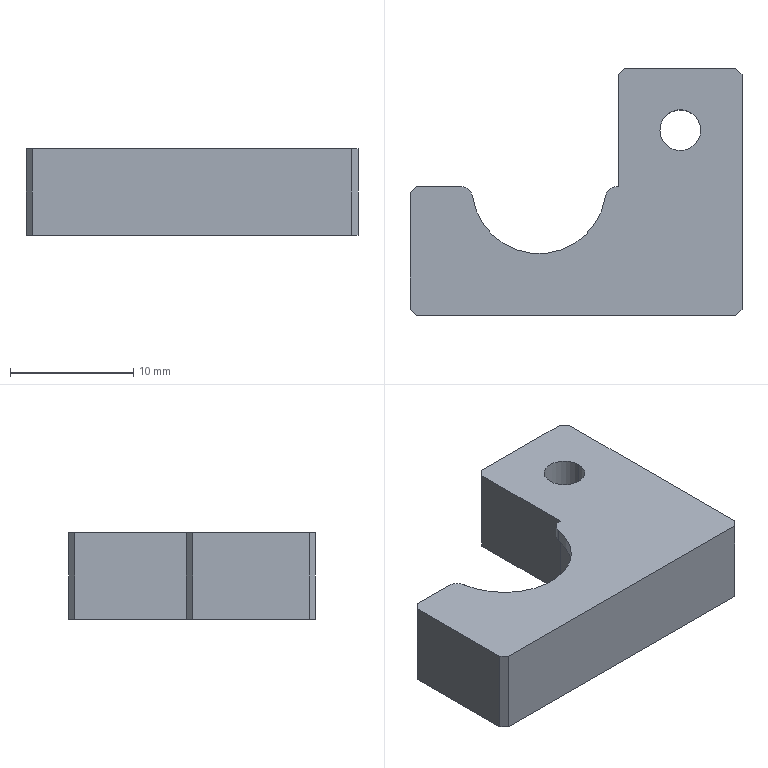Part | SolidWorks | features Chamfer 1, Extrusion 1, Fillet 1, HoleWzd 1, ICE 1 | 1 solid | 22 faces | box 26.9 x 20 x 7 mm | volume 2132 mm3 | plane 16 | cylinder 6 | commonest cylinder face diameters 2 x2 3.3 x2 10.9 x1 12.9 x1
STEP:
#1=CARTESIAN_POINT('',(9.8,4.55,0.));
#2=VERTEX_POINT('',#1);
#3=CARTESIAN_POINT('',(13.1,4.55,0.));
#4=VERTEX_POINT('',#3);
#5=CARTESIAN_POINT('',(11.45,4.55,0.));
#6=DIRECTION('',(0.,0.,1.));
#7=DIRECTION('',(1.,0.,0.));
#8=AXIS2_PLACEMENT_3D('',#5,#6,#7);
#9=CIRCLE('',#8,1.65);
#10=EDGE_CURVE('',#2,#4,#9,.T.);
#11=ORIENTED_EDGE('',*,*,#10,.F.);
#12=CARTESIAN_POINT('',(9.8,4.55,7.));
#13=VERTEX_POINT('',#12);
#14=CARTESIAN_POINT('',(9.8,4.55,7.));
#15=DIRECTION('',(0.,0.,1.));
#16=VECTOR('',#15,1000.);
#17=LINE('',#14,#16);
#18=EDGE_CURVE('',#2,#13,#17,.T.);
#19=ORIENTED_EDGE('',*,*,#18,.T.);
#20=CARTESIAN_POINT('',(13.1,4.55,7.));
#21=VERTEX_POINT('',#20);
#22=CARTESIAN_POINT('',(11.45,4.55,7.));
#23=DIRECTION('',(0.,0.,1.));
#24=DIRECTION('',(1.,0.,0.));
#25=AXIS2_PLACEMENT_3D('',#22,#23,#24);
#26=CIRCLE('',#25,1.65);
#27=EDGE_CURVE('',#13,#21,#26,.T.);
#28=ORIENTED_EDGE('',*,*,#27,.T.);
#29=CARTESIAN_POINT('',(13.1,4.55,7.));
#30=DIRECTION('',(0.,0.,1.));
#31=VECTOR('',#30,1000.);
#32=LINE('',#29,#31);
#33=EDGE_CURVE('',#4,#21,#32,.T.);
#34=ORIENTED_EDGE('',*,*,#33,.F.);
#35=EDGE_LOOP('',(#11,#19,#28,#34));
#36=FACE_OUTER_BOUND('',#35,.T.);
#37=CARTESIAN_POINT('',(11.45,4.55,7.));
#38=DIRECTION('',(0.,0.,1.));
#39=DIRECTION('',(1.,0.,0.));
#40=AXIS2_PLACEMENT_3D('',#37,#38,#39);
#41=CYLINDRICAL_SURFACE('',#40,1.65);
#42=ADVANCED_FACE('',(#36),#41,.F.);
#43=CARTESIAN_POINT('',(6.45,0.,0.));
#44=VERTEX_POINT('',#43);
#45=CARTESIAN_POINT('',(-6.429,-0.5211,0.));
#46=VERTEX_POINT('',#45);
#47=CARTESIAN_POINT('',(0.,0.,0.));
#48=DIRECTION('',(0.,0.,-1.));
#49=DIRECTION('',(1.,0.,0.));
#50=AXIS2_PLACEMENT_3D('',#47,#48,#49);
#51=CIRCLE('',#50,6.45);
#52=EDGE_CURVE('',#44,#46,#51,.T.);
#53=ORIENTED_EDGE('',*,*,#52,.T.);
#54=CARTESIAN_POINT('',(-6.429,-0.5211,6.));
#55=VERTEX_POINT('',#54);
#56=CARTESIAN_POINT('',(-6.429,-0.5211,7.));
#57=DIRECTION('',(0.,0.,1.));
#58=VECTOR('',#57,1000.);
#59=LINE('',#56,#58);
#60=EDGE_CURVE('',#46,#55,#59,.T.);
#61=ORIENTED_EDGE('',*,*,#60,.T.);
#62=CARTESIAN_POINT('',(6.45,0.,6.));
#63=VERTEX_POINT('',#62);
#64=CARTESIAN_POINT('',(0.,0.,6.));
#65=DIRECTION('',(0.,0.,1.));
#66=DIRECTION('',(1.,0.,0.));
#67=AXIS2_PLACEMENT_3D('',#64,#65,#66);
#68=CIRCLE('',#67,6.45);
#69=EDGE_CURVE('',#55,#63,#68,.T.);
#70=ORIENTED_EDGE('',*,*,#69,.T.);
#71=CARTESIAN_POINT('',(6.45,0.,7.));
#72=DIRECTION('',(0.,0.,-1.));
#73=VECTOR('',#72,1000.);
#74=LINE('',#71,#73);
#75=EDGE_CURVE('',#63,#44,#74,.T.);
#76=ORIENTED_EDGE('',*,*,#75,.T.);
#77=EDGE_LOOP('',(#53,#61,#70,#76));
#78=FACE_OUTER_BOUND('',#77,.T.);
#79=CARTESIAN_POINT('',(0.,0.,7.));
#80=DIRECTION('',(0.,0.,-1.));
#81=DIRECTION('',(-1.,0.,0.));
#82=AXIS2_PLACEMENT_3D('',#79,#80,#81);
#83=CYLINDRICAL_SURFACE('',#82,6.45);
#84=ADVANCED_FACE('',(#78),#83,.F.);
#85=CARTESIAN_POINT('',(-6.372,0.,6.));
#86=VERTEX_POINT('',#85);
#87=CARTESIAN_POINT('',(-6.95,0.,6.));
#88=VERTEX_POINT('',#87);
#89=CARTESIAN_POINT('',(-6.45,0.,6.));
#90=DIRECTION('',(-1.,0.,0.));
#91=VECTOR('',#90,1000.);
#92=LINE('',#89,#91);
#93=EDGE_CURVE('',#86,#88,#92,.T.);
#94=ORIENTED_EDGE('',*,*,#93,.T.);
#95=CARTESIAN_POINT('',(-6.95,0.,0.));
#96=VERTEX_POINT('',#95);
#97=CARTESIAN_POINT('',(-6.95,0.,7.));
#98=DIRECTION('',(0.,0.,-1.));
#99=VECTOR('',#98,1000.);
#100=LINE('',#97,#99);
#101=EDGE_CURVE('',#88,#96,#100,.T.);
#102=ORIENTED_EDGE('',*,*,#101,.T.);
#103=CARTESIAN_POINT('',(-9.95,0.,0.));
#104=VERTEX_POINT('',#103);
#105=CARTESIAN_POINT('',(-6.45,0.,0.));
#106=DIRECTION('',(-1.,0.,0.));
#107=VECTOR('',#106,1000.);
#108=LINE('',#105,#107);
#109=EDGE_CURVE('',#96,#104,#108,.T.);
#110=ORIENTED_EDGE('',*,*,#109,.T.);
#111=CARTESIAN_POINT('',(-9.95,0.,7.));
#112=VERTEX_POINT('',#111);
#113=CARTESIAN_POINT('',(-9.95,0.,7.));
#114=DIRECTION('',(0.,0.,1.));
#115=VECTOR('',#114,1000.);
#116=LINE('',#113,#115);
#117=EDGE_CURVE('',#104,#112,#116,.T.);
#118=ORIENTED_EDGE('',*,*,#117,.T.);
#119=CARTESIAN_POINT('',(-6.372,0.,7.));
#120=VERTEX_POINT('',#119);
#121=CARTESIAN_POINT('',(-6.45,0.,7.));
#122=DIRECTION('',(-1.,0.,0.));
#123=VECTOR('',#122,1000.);
#124=LINE('',#121,#123);
#125=EDGE_CURVE('',#120,#112,#124,.T.);
#126=ORIENTED_EDGE('',*,*,#125,.F.);
#127=CARTESIAN_POINT('',(-6.372,0.,6.));
#128=DIRECTION('',(0.,0.,-1.));
#129=VECTOR('',#128,1000.);
#130=LINE('',#127,#129);
#131=EDGE_CURVE('',#120,#86,#130,.T.);
#132=ORIENTED_EDGE('',*,*,#131,.T.);
#133=EDGE_LOOP('',(#94,#102,#110,#118,#126,#132));
#134=FACE_OUTER_BOUND('',#133,.T.);
#135=CARTESIAN_POINT('',(-6.45,0.,7.));
#136=DIRECTION('',(0.,-1.,0.));
#137=DIRECTION('',(1.,0.,0.));
#138=AXIS2_PLACEMENT_3D('',#135,#136,#137);
#139=PLANE('',#138);
#140=ADVANCED_FACE('',(#134),#139,.F.);
#141=CARTESIAN_POINT('',(-10.45,-0.5,0.));
#142=VERTEX_POINT('',#141);
#143=CARTESIAN_POINT('',(-10.45,-9.95,0.));
#144=VERTEX_POINT('',#143);
#145=CARTESIAN_POINT('',(-10.45,0.,0.));
#146=DIRECTION('',(0.,-1.,0.));
#147=VECTOR('',#146,1000.);
#148=LINE('',#145,#147);
#149=EDGE_CURVE('',#142,#144,#148,.T.);
#150=ORIENTED_EDGE('',*,*,#149,.T.);
#151=CARTESIAN_POINT('',(-10.45,-9.95,7.));
#152=VERTEX_POINT('',#151);
#153=CARTESIAN_POINT('',(-10.45,-9.95,7.));
#154=DIRECTION('',(0.,0.,1.));
#155=VECTOR('',#154,1000.);
#156=LINE('',#153,#155);
#157=EDGE_CURVE('',#144,#152,#156,.T.);
#158=ORIENTED_EDGE('',*,*,#157,.T.);
#159=CARTESIAN_POINT('',(-10.45,-0.5,7.));
#160=VERTEX_POINT('',#159);
#161=CARTESIAN_POINT('',(-10.45,0.,7.));
#162=DIRECTION('',(0.,-1.,0.));
#163=VECTOR('',#162,1000.);
#164=LINE('',#161,#163);
#165=EDGE_CURVE('',#160,#152,#164,.T.);
#166=ORIENTED_EDGE('',*,*,#165,.F.);
#167=CARTESIAN_POINT('',(-10.45,-0.5,7.));
#168=DIRECTION('',(0.,0.,-1.));
#169=VECTOR('',#168,1000.);
#170=LINE('',#167,#169);
#171=EDGE_CURVE('',#160,#142,#170,.T.);
#172=ORIENTED_EDGE('',*,*,#171,.T.);
#173=EDGE_LOOP('',(#150,#158,#166,#172));
#174=FACE_OUTER_BOUND('',#173,.T.);
#175=CARTESIAN_POINT('',(-10.45,0.,7.));
#176=DIRECTION('',(1.,0.,0.));
#177=DIRECTION('',(0.,1.,0.));
#178=AXIS2_PLACEMENT_3D('',#175,#176,#177);
#179=PLANE('',#178);
#180=ADVANCED_FACE('',(#174),#179,.F.);
#181=CARTESIAN_POINT('',(-9.95,-10.45,0.));
#182=VERTEX_POINT('',#181);
#183=CARTESIAN_POINT('',(15.95,-10.45,0.));
#184=VERTEX_POINT('',#183);
#185=CARTESIAN_POINT('',(-10.45,-10.45,0.));
#186=DIRECTION('',(1.,0.,0.));
#187=VECTOR('',#186,1000.);
#188=LINE('',#185,#187);
#189=EDGE_CURVE('',#182,#184,#188,.T.);
#190=ORIENTED_EDGE('',*,*,#189,.T.);
#191=CARTESIAN_POINT('',(15.95,-10.45,7.));
#192=VERTEX_POINT('',#191);
#193=CARTESIAN_POINT('',(15.95,-10.45,7.));
#194=DIRECTION('',(0.,0.,1.));
#195=VECTOR('',#194,1000.);
#196=LINE('',#193,#195);
#197=EDGE_CURVE('',#184,#192,#196,.T.);
#198=ORIENTED_EDGE('',*,*,#197,.T.);
#199=CARTESIAN_POINT('',(-9.95,-10.45,7.));
#200=VERTEX_POINT('',#199);
#201=CARTESIAN_POINT('',(-10.45,-10.45,7.));
#202=DIRECTION('',(1.,0.,0.));
#203=VECTOR('',#202,1000.);
#204=LINE('',#201,#203);
#205=EDGE_CURVE('',#200,#192,#204,.T.);
#206=ORIENTED_EDGE('',*,*,#205,.F.);
#207=CARTESIAN_POINT('',(-9.95,-10.45,7.));
#208=DIRECTION('',(0.,0.,-1.));
#209=VECTOR('',#208,1000.);
#210=LINE('',#207,#209);
#211=EDGE_CURVE('',#200,#182,#210,.T.);
#212=ORIENTED_EDGE('',*,*,#211,.T.);
#213=EDGE_LOOP('',(#190,#198,#206,#212));
#214=FACE_OUTER_BOUND('',#213,.T.);
#215=CARTESIAN_POINT('',(-10.45,-10.45,7.));
#216=DIRECTION('',(0.,1.,0.));
#217=DIRECTION('',(0.,0.,1.));
#218=AXIS2_PLACEMENT_3D('',#215,#216,#217);
#219=PLANE('',#218);
#220=ADVANCED_FACE('',(#214),#219,.F.);
#221=CARTESIAN_POINT('',(16.45,-9.95,0.));
#222=VERTEX_POINT('',#221);
#223=CARTESIAN_POINT('',(16.45,9.05,0.));
#224=VERTEX_POINT('',#223);
#225=CARTESIAN_POINT('',(16.45,-10.45,0.));
#226=DIRECTION('',(0.,1.,0.));
#227=VECTOR('',#226,1000.);
#228=LINE('',#225,#227);
#229=EDGE_CURVE('',#222,#224,#228,.T.);
#230=ORIENTED_EDGE('',*,*,#229,.T.);
#231=CARTESIAN_POINT('',(16.45,9.05,7.));
#232=VERTEX_POINT('',#231);
#233=CARTESIAN_POINT('',(16.45,9.05,7.));
#234=DIRECTION('',(0.,0.,1.));
#235=VECTOR('',#234,1000.);
#236=LINE('',#233,#235);
#237=EDGE_CURVE('',#224,#232,#236,.T.);
#238=ORIENTED_EDGE('',*,*,#237,.T.);
#239=CARTESIAN_POINT('',(16.45,-9.95,7.));
#240=VERTEX_POINT('',#239);
#241=CARTESIAN_POINT('',(16.45,-10.45,7.));
#242=DIRECTION('',(0.,1.,0.));
#243=VECTOR('',#242,1000.);
#244=LINE('',#241,#243);
#245=EDGE_CURVE('',#240,#232,#244,.T.);
#246=ORIENTED_EDGE('',*,*,#245,.F.);
#247=CARTESIAN_POINT('',(16.45,-9.95,7.));
#248=DIRECTION('',(0.,0.,-1.));
#249=VECTOR('',#248,1000.);
#250=LINE('',#247,#249);
#251=EDGE_CURVE('',#240,#222,#250,.T.);
#252=ORIENTED_EDGE('',*,*,#251,.T.);
#253=EDGE_LOOP('',(#230,#238,#246,#252));
#254=FACE_OUTER_BOUND('',#253,.T.);
#255=CARTESIAN_POINT('',(16.45,-10.45,7.));
#256=DIRECTION('',(-1.,0.,0.));
#257=DIRECTION('',(0.,0.,1.));
#258=AXIS2_PLACEMENT_3D('',#255,#256,#257);
#259=PLANE('',#258);
#260=ADVANCED_FACE('',(#254),#259,.F.);
#261=CARTESIAN_POINT('',(15.95,9.55,7.));
#262=VERTEX_POINT('',#261);
#263=CARTESIAN_POINT('',(6.95,9.55,7.));
#264=VERTEX_POINT('',#263);
#265=CARTESIAN_POINT('',(16.45,9.55,7.));
#266=DIRECTION('',(-1.,0.,0.));
#267=VECTOR('',#266,1000.);
#268=LINE('',#265,#267);
#269=EDGE_CURVE('',#262,#264,#268,.T.);
#270=ORIENTED_EDGE('',*,*,#269,.F.);
#271=CARTESIAN_POINT('',(15.95,9.55,0.));
#272=VERTEX_POINT('',#271);
#273=CARTESIAN_POINT('',(15.95,9.55,7.));
#274=DIRECTION('',(0.,0.,-1.));
#275=VECTOR('',#274,1000.);
#276=LINE('',#273,#275);
#277=EDGE_CURVE('',#262,#272,#276,.T.);
#278=ORIENTED_EDGE('',*,*,#277,.T.);
#279=CARTESIAN_POINT('',(6.95,9.55,0.));
#280=VERTEX_POINT('',#279);
#281=CARTESIAN_POINT('',(16.45,9.55,0.));
#282=DIRECTION('',(-1.,0.,0.));
#283=VECTOR('',#282,1000.);
#284=LINE('',#281,#283);
#285=EDGE_CURVE('',#272,#280,#284,.T.);
#286=ORIENTED_EDGE('',*,*,#285,.T.);
#287=CARTESIAN_POINT('',(6.95,9.55,7.));
#288=DIRECTION('',(0.,0.,1.));
#289=VECTOR('',#288,1000.);
#290=LINE('',#287,#289);
#291=EDGE_CURVE('',#280,#264,#290,.T.);
#292=ORIENTED_EDGE('',*,*,#291,.T.);
#293=EDGE_LOOP('',(#270,#278,#286,#292));
#294=FACE_OUTER_BOUND('',#293,.T.);
#295=CARTESIAN_POINT('',(16.45,9.55,7.));
#296=DIRECTION('',(0.,-1.,0.));
#297=DIRECTION('',(1.,0.,0.));
#298=AXIS2_PLACEMENT_3D('',#295,#296,#297);
#299=PLANE('',#298);
#300=ADVANCED_FACE('',(#294),#299,.F.);
#301=CARTESIAN_POINT('',(6.45,9.05,7.));
#302=VERTEX_POINT('',#301);
#303=CARTESIAN_POINT('',(6.45,0.,7.));
#304=VERTEX_POINT('',#303);
#305=CARTESIAN_POINT('',(6.45,9.55,7.));
#306=DIRECTION('',(0.,-1.,0.));
#307=VECTOR('',#306,1000.);
#308=LINE('',#305,#307);
#309=EDGE_CURVE('',#302,#304,#308,.T.);
#310=ORIENTED_EDGE('',*,*,#309,.F.);
#311=CARTESIAN_POINT('',(6.45,9.05,0.));
#312=VERTEX_POINT('',#311);
#313=CARTESIAN_POINT('',(6.45,9.05,7.));
#314=DIRECTION('',(0.,0.,-1.));
#315=VECTOR('',#314,1000.);
#316=LINE('',#313,#315);
#317=EDGE_CURVE('',#302,#312,#316,.T.);
#318=ORIENTED_EDGE('',*,*,#317,.T.);
#319=CARTESIAN_POINT('',(6.45,9.55,0.));
#320=DIRECTION('',(0.,-1.,0.));
#321=VECTOR('',#320,1000.);
#322=LINE('',#319,#321);
#323=EDGE_CURVE('',#312,#44,#322,.T.);
#324=ORIENTED_EDGE('',*,*,#323,.T.);
#325=ORIENTED_EDGE('',*,*,#75,.F.);
#326=CARTESIAN_POINT('',(6.45,0.,7.));
#327=DIRECTION('',(0.,0.,-1.));
#328=VECTOR('',#327,1000.);
#329=LINE('',#326,#328);
#330=EDGE_CURVE('',#304,#63,#329,.T.);
#331=ORIENTED_EDGE('',*,*,#330,.F.);
#332=EDGE_LOOP('',(#310,#318,#324,#325,#331));
#333=FACE_OUTER_BOUND('',#332,.T.);
#334=CARTESIAN_POINT('',(6.45,9.55,7.));
#335=DIRECTION('',(1.,0.,0.));
#336=DIRECTION('',(0.,0.,-1.));
#337=AXIS2_PLACEMENT_3D('',#334,#335,#336);
#338=PLANE('',#337);
#339=ADVANCED_FACE('',(#333),#338,.F.);
#340=CARTESIAN_POINT('',(11.45,4.55,7.));
#341=DIRECTION('',(0.,0.,1.));
#342=DIRECTION('',(1.,0.,0.));
#343=AXIS2_PLACEMENT_3D('',#340,#341,#342);
#344=CIRCLE('',#343,1.65);
#345=EDGE_CURVE('',#21,#13,#344,.T.);
#346=ORIENTED_EDGE('',*,*,#345,.F.);
#347=ORIENTED_EDGE('',*,*,#27,.F.);
#348=EDGE_LOOP('',(#346,#347));
#349=FACE_BOUND('',#348,.T.);
#350=ORIENTED_EDGE('',*,*,#245,.T.);
#351=CARTESIAN_POINT('',(12.75,12.75,7.));
#352=DIRECTION('',(-0.7071,0.7071,0.));
#353=VECTOR('',#352,1000.);
#354=LINE('',#351,#353);
#355=EDGE_CURVE('',#232,#262,#354,.T.);
#356=ORIENTED_EDGE('',*,*,#355,.T.);
#357=ORIENTED_EDGE('',*,*,#269,.T.);
#358=CARTESIAN_POINT('',(-1.3,1.3,7.));
#359=DIRECTION('',(-0.7071,-0.7071,0.));
#360=VECTOR('',#359,1000.);
#361=LINE('',#358,#360);
#362=EDGE_CURVE('',#264,#302,#361,.T.);
#363=ORIENTED_EDGE('',*,*,#362,.T.);
#364=ORIENTED_EDGE('',*,*,#309,.T.);
#365=CARTESIAN_POINT('',(6.372,0.,7.));
#366=VERTEX_POINT('',#365);
#367=CARTESIAN_POINT('',(5.45,0.,7.));
#368=DIRECTION('',(-1.,0.,0.));
#369=VECTOR('',#368,1000.);
#370=LINE('',#367,#369);
#371=EDGE_CURVE('',#304,#366,#370,.T.);
#372=ORIENTED_EDGE('',*,*,#371,.T.);
#373=CARTESIAN_POINT('',(5.384,-0.845,7.));
#374=VERTEX_POINT('',#373);
#375=CARTESIAN_POINT('',(6.372,-1.,7.));
#376=DIRECTION('',(0.,0.,1.));
#377=DIRECTION('',(1.,0.,0.));
#378=AXIS2_PLACEMENT_3D('',#375,#376,#377);
#379=CIRCLE('',#378,1.);
#380=EDGE_CURVE('',#366,#374,#379,.T.);
#381=ORIENTED_EDGE('',*,*,#380,.T.);
#382=CARTESIAN_POINT('',(-5.384,-0.845,7.));
#383=VERTEX_POINT('',#382);
#384=CARTESIAN_POINT('',(0.,0.,7.));
#385=DIRECTION('',(0.,0.,-1.));
#386=DIRECTION('',(1.,0.,0.));
#387=AXIS2_PLACEMENT_3D('',#384,#385,#386);
#388=CIRCLE('',#387,5.45);
#389=EDGE_CURVE('',#374,#383,#388,.T.);
#390=ORIENTED_EDGE('',*,*,#389,.T.);
#391=CARTESIAN_POINT('',(-6.372,-1.,7.));
#392=DIRECTION('',(0.,0.,1.));
#393=DIRECTION('',(1.,0.,0.));
#394=AXIS2_PLACEMENT_3D('',#391,#392,#393);
#395=CIRCLE('',#394,1.);
#396=EDGE_CURVE('',#383,#120,#395,.T.);
#397=ORIENTED_EDGE('',*,*,#396,.T.);
#398=ORIENTED_EDGE('',*,*,#125,.T.);
#399=CARTESIAN_POINT('',(-4.975,4.975,7.));
#400=DIRECTION('',(-0.7071,-0.7071,0.));
#401=VECTOR('',#400,1000.);
#402=LINE('',#399,#401);
#403=EDGE_CURVE('',#112,#160,#402,.T.);
#404=ORIENTED_EDGE('',*,*,#403,.T.);
#405=ORIENTED_EDGE('',*,*,#165,.T.);
#406=CARTESIAN_POINT('',(-10.2,-10.2,7.));
#407=DIRECTION('',(0.7071,-0.7071,0.));
#408=VECTOR('',#407,1000.);
#409=LINE('',#406,#408);
#410=EDGE_CURVE('',#152,#200,#409,.T.);
#411=ORIENTED_EDGE('',*,*,#410,.T.);
#412=ORIENTED_EDGE('',*,*,#205,.T.);
#413=CARTESIAN_POINT('',(13.2,-13.2,7.));
#414=DIRECTION('',(0.7071,0.7071,0.));
#415=VECTOR('',#414,1000.);
#416=LINE('',#413,#415);
#417=EDGE_CURVE('',#192,#240,#416,.T.);
#418=ORIENTED_EDGE('',*,*,#417,.T.);
#419=EDGE_LOOP('',(#350,#356,#357,#363,#364,#372,#381,#390,#397,#398,#404,#405,#411,#412,#418));
#420=FACE_OUTER_BOUND('',#419,.T.);
#421=CARTESIAN_POINT('',(0.,0.,7.));
#422=DIRECTION('',(0.,0.,1.));
#423=DIRECTION('',(1.,0.,0.));
#424=AXIS2_PLACEMENT_3D('',#421,#422,#423);
#425=PLANE('',#424);
#426=ADVANCED_FACE('',(#349,#420),#425,.T.);
#427=CARTESIAN_POINT('',(11.45,4.55,0.));
#428=DIRECTION('',(0.,0.,1.));
#429=DIRECTION('',(1.,0.,0.));
#430=AXIS2_PLACEMENT_3D('',#427,#428,#429);
#431=CIRCLE('',#430,1.65);
#432=EDGE_CURVE('',#4,#2,#431,.T.);
#433=ORIENTED_EDGE('',*,*,#432,.T.);
#434=ORIENTED_EDGE('',*,*,#10,.T.);
#435=EDGE_LOOP('',(#433,#434));
#436=FACE_BOUND('',#435,.T.);
#437=ORIENTED_EDGE('',*,*,#285,.F.);
#438=CARTESIAN_POINT('',(15.95,9.55,0.));
#439=DIRECTION('',(0.7071,-0.7071,0.));
#440=VECTOR('',#439,1000.);
#441=LINE('',#438,#440);
#442=EDGE_CURVE('',#272,#224,#441,.T.);
#443=ORIENTED_EDGE('',*,*,#442,.T.);
#444=ORIENTED_EDGE('',*,*,#229,.F.);
#445=CARTESIAN_POINT('',(16.45,-9.95,0.));
#446=DIRECTION('',(-0.7071,-0.7071,0.));
#447=VECTOR('',#446,1000.);
#448=LINE('',#445,#447);
#449=EDGE_CURVE('',#222,#184,#448,.T.);
#450=ORIENTED_EDGE('',*,*,#449,.T.);
#451=ORIENTED_EDGE('',*,*,#189,.F.);
#452=CARTESIAN_POINT('',(-9.95,-10.45,0.));
#453=DIRECTION('',(-0.7071,0.7071,0.));
#454=VECTOR('',#453,1000.);
#455=LINE('',#452,#454);
#456=EDGE_CURVE('',#182,#144,#455,.T.);
#457=ORIENTED_EDGE('',*,*,#456,.T.);
#458=ORIENTED_EDGE('',*,*,#149,.F.);
#459=CARTESIAN_POINT('',(-10.45,-0.5,0.));
#460=DIRECTION('',(0.7071,0.7071,0.));
#461=VECTOR('',#460,1000.);
#462=LINE('',#459,#461);
#463=EDGE_CURVE('',#142,#104,#462,.T.);
#464=ORIENTED_EDGE('',*,*,#463,.T.);
#465=ORIENTED_EDGE('',*,*,#109,.F.);
#466=CARTESIAN_POINT('',(-6.95,0.,0.));
#467=DIRECTION('',(0.7071,-0.7071,0.));
#468=VECTOR('',#467,1000.);
#469=LINE('',#466,#468);
#470=EDGE_CURVE('',#96,#46,#469,.T.);
#471=ORIENTED_EDGE('',*,*,#470,.T.);
#472=ORIENTED_EDGE('',*,*,#52,.F.);
#473=ORIENTED_EDGE('',*,*,#323,.F.);
#474=CARTESIAN_POINT('',(6.45,9.05,0.));
#475=DIRECTION('',(0.7071,0.7071,0.));
#476=VECTOR('',#475,1000.);
#477=LINE('',#474,#476);
#478=EDGE_CURVE('',#312,#280,#477,.T.);
#479=ORIENTED_EDGE('',*,*,#478,.T.);
#480=EDGE_LOOP('',(#437,#443,#444,#450,#451,#457,#458,#464,#465,#471,#472,#473,#479));
#481=FACE_OUTER_BOUND('',#480,.T.);
#482=CARTESIAN_POINT('',(0.,0.,0.));
#483=DIRECTION('',(0.,0.,1.));
#484=DIRECTION('',(1.,0.,0.));
#485=AXIS2_PLACEMENT_3D('',#482,#483,#484);
#486=PLANE('',#485);
#487=ADVANCED_FACE('',(#436,#481),#486,.F.);
#488=ORIENTED_EDGE('',*,*,#18,.F.);
#489=ORIENTED_EDGE('',*,*,#432,.F.);
#490=ORIENTED_EDGE('',*,*,#33,.T.);
#491=ORIENTED_EDGE('',*,*,#345,.T.);
#492=EDGE_LOOP('',(#488,#489,#490,#491));
#493=FACE_OUTER_BOUND('',#492,.T.);
#494=CARTESIAN_POINT('',(11.45,4.55,7.));
#495=DIRECTION('',(0.,0.,1.));
#496=DIRECTION('',(1.,0.,0.));
#497=AXIS2_PLACEMENT_3D('',#494,#495,#496);
#498=CYLINDRICAL_SURFACE('',#497,1.65);
#499=ADVANCED_FACE('',(#493),#498,.F.);
#500=ORIENTED_EDGE('',*,*,#389,.F.);
#501=CARTESIAN_POINT('',(5.384,-0.845,6.));
#502=VERTEX_POINT('',#501);
#503=CARTESIAN_POINT('',(5.384,-0.845,6.));
#504=DIRECTION('',(0.,0.,-1.));
#505=VECTOR('',#504,1000.);
#506=LINE('',#503,#505);
#507=EDGE_CURVE('',#374,#502,#506,.T.);
#508=ORIENTED_EDGE('',*,*,#507,.T.);
#509=CARTESIAN_POINT('',(-5.384,-0.845,6.));
#510=VERTEX_POINT('',#509);
#511=CARTESIAN_POINT('',(0.,0.,6.));
#512=DIRECTION('',(0.,0.,-1.));
#513=DIRECTION('',(1.,0.,0.));
#514=AXIS2_PLACEMENT_3D('',#511,#512,#513);
#515=CIRCLE('',#514,5.45);
#516=EDGE_CURVE('',#502,#510,#515,.T.);
#517=ORIENTED_EDGE('',*,*,#516,.T.);
#518=CARTESIAN_POINT('',(-5.384,-0.845,6.));
#519=DIRECTION('',(0.,0.,1.));
#520=VECTOR('',#519,1000.);
#521=LINE('',#518,#520);
#522=EDGE_CURVE('',#510,#383,#521,.T.);
#523=ORIENTED_EDGE('',*,*,#522,.T.);
#524=EDGE_LOOP('',(#500,#508,#517,#523));
#525=FACE_OUTER_BOUND('',#524,.T.);
#526=CARTESIAN_POINT('',(0.,0.,6.));
#527=DIRECTION('',(0.,0.,1.));
#528=DIRECTION('',(1.,0.,0.));
#529=AXIS2_PLACEMENT_3D('',#526,#527,#528);
#530=CYLINDRICAL_SURFACE('',#529,5.45);
#531=ADVANCED_FACE('',(#525),#530,.F.);
#532=CARTESIAN_POINT('',(6.372,0.,6.));
#533=VERTEX_POINT('',#532);
#534=CARTESIAN_POINT('',(5.45,0.,6.));
#535=DIRECTION('',(-1.,0.,0.));
#536=VECTOR('',#535,1000.);
#537=LINE('',#534,#536);
#538=EDGE_CURVE('',#63,#533,#537,.T.);
#539=ORIENTED_EDGE('',*,*,#538,.T.);
#540=CARTESIAN_POINT('',(6.372,0.,6.));
#541=DIRECTION('',(0.,0.,1.));
#542=VECTOR('',#541,1000.);
#543=LINE('',#540,#542);
#544=EDGE_CURVE('',#533,#366,#543,.T.);
#545=ORIENTED_EDGE('',*,*,#544,.T.);
#546=ORIENTED_EDGE('',*,*,#371,.F.);
#547=ORIENTED_EDGE('',*,*,#330,.T.);
#548=EDGE_LOOP('',(#539,#545,#546,#547));
#549=FACE_OUTER_BOUND('',#548,.T.);
#550=CARTESIAN_POINT('',(5.45,0.,6.));
#551=DIRECTION('',(0.,1.,0.));
#552=DIRECTION('',(-1.,0.,0.));
#553=AXIS2_PLACEMENT_3D('',#550,#551,#552);
#554=PLANE('',#553);
#555=ADVANCED_FACE('',(#549),#554,.T.);
#556=ORIENTED_EDGE('',*,*,#516,.F.);
#557=CARTESIAN_POINT('',(6.372,-1.,6.));
#558=DIRECTION('',(0.,0.,-1.));
#559=DIRECTION('',(1.,0.,0.));
#560=AXIS2_PLACEMENT_3D('',#557,#558,#559);
#561=CIRCLE('',#560,1.);
#562=EDGE_CURVE('',#502,#533,#561,.T.);
#563=ORIENTED_EDGE('',*,*,#562,.T.);
#564=ORIENTED_EDGE('',*,*,#538,.F.);
#565=ORIENTED_EDGE('',*,*,#69,.F.);
#566=CARTESIAN_POINT('',(-3.475,-3.475,6.));
#567=DIRECTION('',(-0.7071,0.7071,0.));
#568=VECTOR('',#567,1000.);
#569=LINE('',#566,#568);
#570=EDGE_CURVE('',#55,#88,#569,.T.);
#571=ORIENTED_EDGE('',*,*,#570,.T.);
#572=ORIENTED_EDGE('',*,*,#93,.F.);
#573=CARTESIAN_POINT('',(-6.372,-1.,6.));
#574=DIRECTION('',(0.,0.,-1.));
#575=DIRECTION('',(1.,0.,0.));
#576=AXIS2_PLACEMENT_3D('',#573,#574,#575);
#577=CIRCLE('',#576,1.);
#578=EDGE_CURVE('',#86,#510,#577,.T.);
#579=ORIENTED_EDGE('',*,*,#578,.T.);
#580=EDGE_LOOP('',(#556,#563,#564,#565,#571,#572,#579));
#581=FACE_OUTER_BOUND('',#580,.T.);
#582=CARTESIAN_POINT('',(0.,0.,6.));
#583=DIRECTION('',(0.,0.,1.));
#584=DIRECTION('',(1.,0.,0.));
#585=AXIS2_PLACEMENT_3D('',#582,#583,#584);
#586=PLANE('',#585);
#587=ADVANCED_FACE('',(#581),#586,.F.);
#588=ORIENTED_EDGE('',*,*,#562,.F.);
#589=ORIENTED_EDGE('',*,*,#507,.F.);
#590=ORIENTED_EDGE('',*,*,#380,.F.);
#591=ORIENTED_EDGE('',*,*,#544,.F.);
#592=EDGE_LOOP('',(#588,#589,#590,#591));
#593=FACE_OUTER_BOUND('',#592,.T.);
#594=CARTESIAN_POINT('',(6.372,-1.,6.));
#595=DIRECTION('',(0.,0.,1.));
#596=DIRECTION('',(1.,0.,0.));
#597=AXIS2_PLACEMENT_3D('',#594,#595,#596);
#598=CYLINDRICAL_SURFACE('',#597,1.);
#599=ADVANCED_FACE('',(#593),#598,.T.);
#600=ORIENTED_EDGE('',*,*,#578,.F.);
#601=ORIENTED_EDGE('',*,*,#131,.F.);
#602=ORIENTED_EDGE('',*,*,#396,.F.);
#603=ORIENTED_EDGE('',*,*,#522,.F.);
#604=EDGE_LOOP('',(#600,#601,#602,#603));
#605=FACE_OUTER_BOUND('',#604,.T.);
#606=CARTESIAN_POINT('',(-6.372,-1.,6.));
#607=DIRECTION('',(0.,0.,1.));
#608=DIRECTION('',(1.,0.,0.));
#609=AXIS2_PLACEMENT_3D('',#606,#607,#608);
#610=CYLINDRICAL_SURFACE('',#609,1.);
#611=ADVANCED_FACE('',(#605),#610,.T.);
#612=ORIENTED_EDGE('',*,*,#355,.F.);
#613=ORIENTED_EDGE('',*,*,#237,.F.);
#614=ORIENTED_EDGE('',*,*,#442,.F.);
#615=ORIENTED_EDGE('',*,*,#277,.F.);
#616=EDGE_LOOP('',(#612,#613,#614,#615));
#617=FACE_OUTER_BOUND('',#616,.T.);
#618=CARTESIAN_POINT('',(15.95,9.55,7.));
#619=DIRECTION('',(-0.7071,-0.7071,0.));
#620=DIRECTION('',(0.,0.,-1.));
#621=AXIS2_PLACEMENT_3D('',#618,#619,#620);
#622=PLANE('',#621);
#623=ADVANCED_FACE('',(#617),#622,.F.);
#624=ORIENTED_EDGE('',*,*,#417,.F.);
#625=ORIENTED_EDGE('',*,*,#197,.F.);
#626=ORIENTED_EDGE('',*,*,#449,.F.);
#627=ORIENTED_EDGE('',*,*,#251,.F.);
#628=EDGE_LOOP('',(#624,#625,#626,#627));
#629=FACE_OUTER_BOUND('',#628,.T.);
#630=CARTESIAN_POINT('',(16.45,-9.95,7.));
#631=DIRECTION('',(-0.7071,0.7071,0.));
#632=DIRECTION('',(0.,0.,-1.));
#633=AXIS2_PLACEMENT_3D('',#630,#631,#632);
#634=PLANE('',#633);
#635=ADVANCED_FACE('',(#629),#634,.F.);
#636=ORIENTED_EDGE('',*,*,#410,.F.);
#637=ORIENTED_EDGE('',*,*,#157,.F.);
#638=ORIENTED_EDGE('',*,*,#456,.F.);
#639=ORIENTED_EDGE('',*,*,#211,.F.);
#640=EDGE_LOOP('',(#636,#637,#638,#639));
#641=FACE_OUTER_BOUND('',#640,.T.);
#642=CARTESIAN_POINT('',(-9.95,-10.45,7.));
#643=DIRECTION('',(0.7071,0.7071,0.));
#644=DIRECTION('',(0.,0.,-1.));
#645=AXIS2_PLACEMENT_3D('',#642,#643,#644);
#646=PLANE('',#645);
#647=ADVANCED_FACE('',(#641),#646,.F.);
#648=ORIENTED_EDGE('',*,*,#362,.F.);
#649=ORIENTED_EDGE('',*,*,#291,.F.);
#650=ORIENTED_EDGE('',*,*,#478,.F.);
#651=ORIENTED_EDGE('',*,*,#317,.F.);
#652=EDGE_LOOP('',(#648,#649,#650,#651));
#653=FACE_OUTER_BOUND('',#652,.T.);
#654=CARTESIAN_POINT('',(6.45,9.05,7.));
#655=DIRECTION('',(0.7071,-0.7071,0.));
#656=DIRECTION('',(0.,0.,-1.));
#657=AXIS2_PLACEMENT_3D('',#654,#655,#656);
#658=PLANE('',#657);
#659=ADVANCED_FACE('',(#653),#658,.F.);
#660=ORIENTED_EDGE('',*,*,#570,.F.);
#661=ORIENTED_EDGE('',*,*,#60,.F.);
#662=ORIENTED_EDGE('',*,*,#470,.F.);
#663=ORIENTED_EDGE('',*,*,#101,.F.);
#664=EDGE_LOOP('',(#660,#661,#662,#663));
#665=FACE_OUTER_BOUND('',#664,.T.);
#666=CARTESIAN_POINT('',(-6.95,0.,7.));
#667=DIRECTION('',(-0.7071,-0.7071,0.));
#668=DIRECTION('',(0.,0.,-1.));
#669=AXIS2_PLACEMENT_3D('',#666,#667,#668);
#670=PLANE('',#669);
#671=ADVANCED_FACE('',(#665),#670,.F.);
#672=ORIENTED_EDGE('',*,*,#403,.F.);
#673=ORIENTED_EDGE('',*,*,#117,.F.);
#674=ORIENTED_EDGE('',*,*,#463,.F.);
#675=ORIENTED_EDGE('',*,*,#171,.F.);
#676=EDGE_LOOP('',(#672,#673,#674,#675));
#677=FACE_OUTER_BOUND('',#676,.T.);
#678=CARTESIAN_POINT('',(-10.45,-0.5,7.));
#679=DIRECTION('',(0.7071,-0.7071,0.));
#680=DIRECTION('',(0.,0.,-1.));
#681=AXIS2_PLACEMENT_3D('',#678,#679,#680);
#682=PLANE('',#681);
#683=ADVANCED_FACE('',(#677),#682,.F.);
#684=CLOSED_SHELL('',(#42,#84,#140,#180,#220,#260,#300,#339,#426,#487,#499,#531,#555,#587,#599,#611,#623,#635,#647,#659,#671,#683));
#685=MANIFOLD_SOLID_BREP('',#684);
#686=CARTESIAN_POINT('',(0.,0.,0.));
#687=DIRECTION('',(0.,0.,1.));
#688=DIRECTION('',(1.,0.,0.));
#689=AXIS2_PLACEMENT_3D('',#686,#687,#688);
#690=(LENGTH_UNIT()NAMED_UNIT(*)SI_UNIT(.MILLI.,.METRE.));
#691=UNCERTAINTY_MEASURE_WITH_UNIT(LENGTH_MEASURE(0.00001),#690,'','');
#692=(NAMED_UNIT(*)PLANE_ANGLE_UNIT()SI_UNIT($,.RADIAN.));
#693=(NAMED_UNIT(*)SI_UNIT($,.STERADIAN.)SOLID_ANGLE_UNIT());
#694=(GEOMETRIC_REPRESENTATION_CONTEXT(3)GLOBAL_UNCERTAINTY_ASSIGNED_CONTEXT((#691))GLOBAL_UNIT_ASSIGNED_CONTEXT((#690,#692,#693))REPRESENTATION_CONTEXT('',''));
#695=ADVANCED_BREP_SHAPE_REPRESENTATION('',(#685,#689),#694);